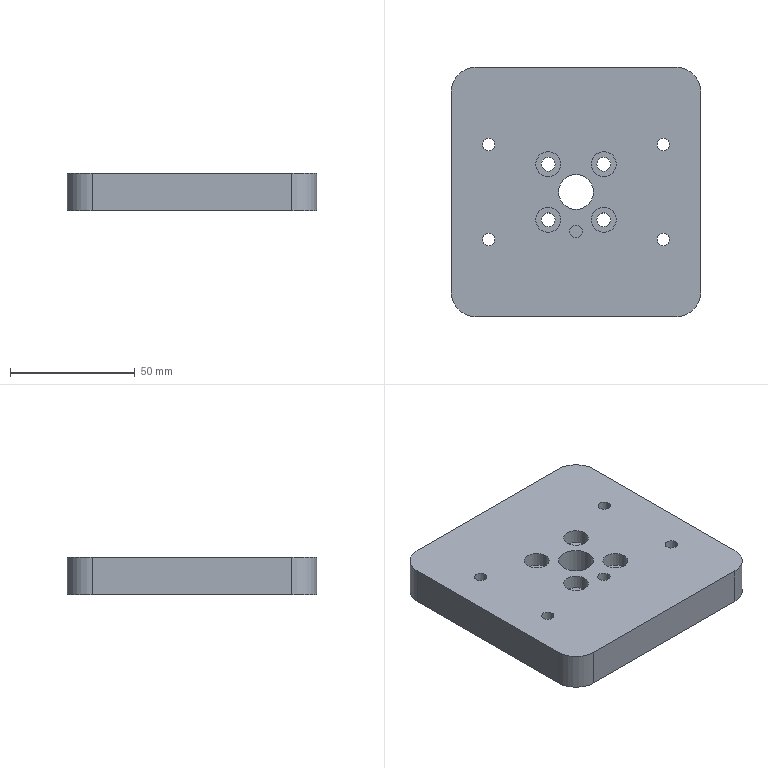NC program | NX | posted with a generic post | part box 100 x 100 x 15 mm
Lines 1 to 24 of 2072:
N10 G17 G21 G94 G90
(FLOOR_WALL_1 , TOOL : D63)
N12 T01 M6
N14 G54
N16 G17 G0 G90 X-86.5 Y51.997 S6500 M3
N18 G43 Z30. H1
N20 Z3.
N22 G94 G1 Z0. F1500.
N24 X-83.5
N26 X83.5
N28 Y25.731
N30 X-83.5
N32 Y-0.534
N34 X83.5
N36 Y-26.8
N38 X-83.5
N40 X-86.5
N42 Z3.
N44 G0 Z30.
N46 M5